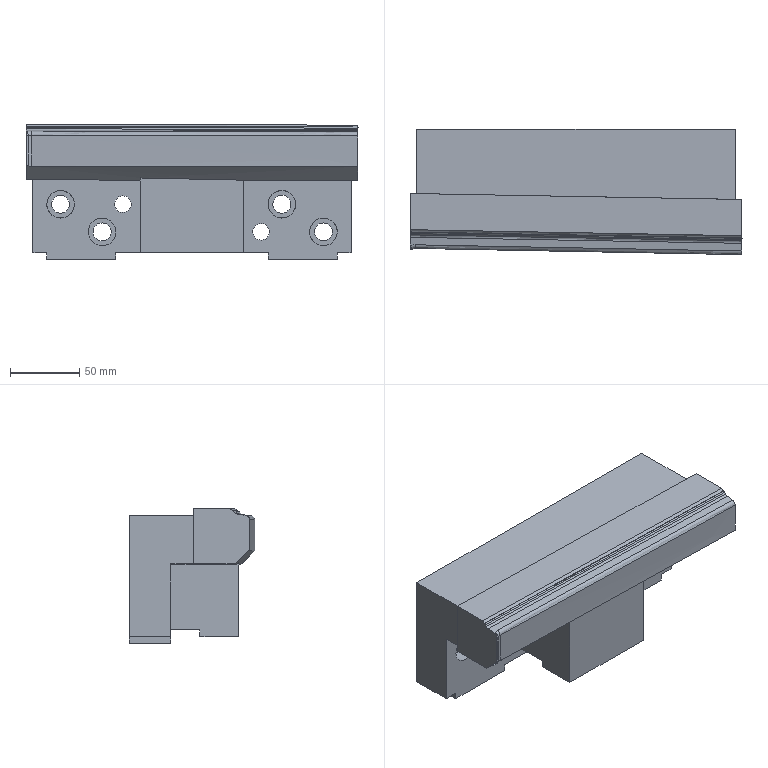Part | NX | features solid 2 | 1 solid | 55 faces | box 240 x 90.564 x 97.69 mm | volume 1277587 mm3 | plane 25 | spline 20 | cylinder 10 | commonest cylinder face diameters 13 x4 20 x4 12 x2